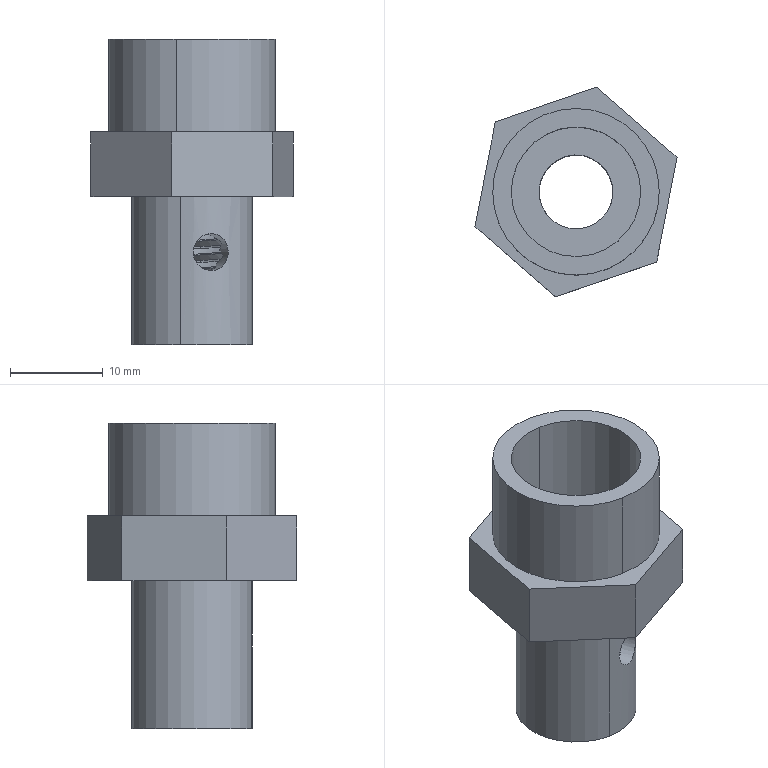Part | SolidWorks | features BaseBody 1 | 1 solid | 76 faces | box 21.836 x 22.67 x 33 mm | volume 4158 mm3 | cylinder 54 | plane 12 | spline 7 | cone 3 | commonest cylinder face diameters 10 x24 8 x22 4 x2 13 x2 14 x2 18 x2